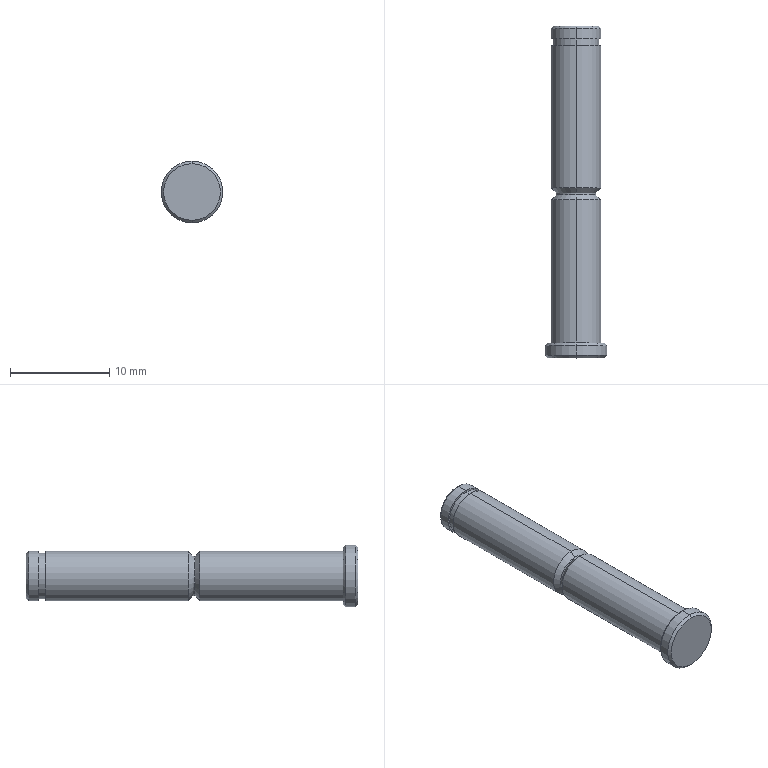Part | NX | features BREP 1 | 1 solid | 27 faces | box 6.2 x 33.4 x 6.2 mm | volume 662.792 mm3 | cylinder 12 | cone 10 | plane 5 | commonest cylinder face diameters 5 x6 4 x2 4.6 x2 6.2 x2
STEP:
#1=CARTESIAN_POINT('',(0.,33.4,2.25));
#2=VERTEX_POINT('',#1);
#3=CARTESIAN_POINT('',(0.,33.15,2.5));
#4=VERTEX_POINT('',#3);
#5=CARTESIAN_POINT('',(0.,33.15,2.5));
#6=DIRECTION('',(0.,-0.7071,0.7071));
#7=VECTOR('',#6,1000.);
#8=LINE('',#5,#7);
#9=EDGE_CURVE('',#2,#4,#8,.T.);
#10=ORIENTED_EDGE('',*,*,#9,.F.);
#11=CARTESIAN_POINT('',(0.,33.4,-2.25));
#12=VERTEX_POINT('',#11);
#13=CARTESIAN_POINT('',(0.,33.4,0.));
#14=DIRECTION('',(0.,1.,0.));
#15=DIRECTION('',(0.,0.,-1.));
#16=AXIS2_PLACEMENT_3D('',#13,#14,#15);
#17=CIRCLE('',#16,2.25);
#18=EDGE_CURVE('',#12,#2,#17,.T.);
#19=ORIENTED_EDGE('',*,*,#18,.F.);
#20=CARTESIAN_POINT('',(0.,33.15,-2.5));
#21=VERTEX_POINT('',#20);
#22=CARTESIAN_POINT('',(0.,33.15,-2.5));
#23=DIRECTION('',(0.,-0.7071,-0.7071));
#24=VECTOR('',#23,1000.);
#25=LINE('',#22,#24);
#26=EDGE_CURVE('',#12,#21,#25,.T.);
#27=ORIENTED_EDGE('',*,*,#26,.T.);
#28=CARTESIAN_POINT('',(0.,33.15,0.));
#29=DIRECTION('',(0.,-1.,0.));
#30=DIRECTION('',(0.,0.,-1.));
#31=AXIS2_PLACEMENT_3D('',#28,#29,#30);
#32=CIRCLE('',#31,2.5);
#33=EDGE_CURVE('',#4,#21,#32,.T.);
#34=ORIENTED_EDGE('',*,*,#33,.F.);
#35=EDGE_LOOP('',(#10,#19,#27,#34));
#36=FACE_BOUND('',#35,.T.);
#37=CARTESIAN_POINT('',(0.,33.15,0.));
#38=DIRECTION('',(0.,-1.,0.));
#39=DIRECTION('',(0.,0.,-1.));
#40=AXIS2_PLACEMENT_3D('',#37,#38,#39);
#41=CONICAL_SURFACE('',#40,2.5,0.7854);
#42=ADVANCED_FACE('',(#36),#41,.T.);
#43=CARTESIAN_POINT('',(0.,1.5,2.85));
#44=VERTEX_POINT('',#43);
#45=CARTESIAN_POINT('',(0.,1.25,3.1));
#46=VERTEX_POINT('',#45);
#47=CARTESIAN_POINT('',(0.,1.25,3.1));
#48=DIRECTION('',(0.,-0.7071,0.7071));
#49=VECTOR('',#48,1000.);
#50=LINE('',#47,#49);
#51=EDGE_CURVE('',#44,#46,#50,.T.);
#52=ORIENTED_EDGE('',*,*,#51,.F.);
#53=CARTESIAN_POINT('',(0.,1.5,-2.85));
#54=VERTEX_POINT('',#53);
#55=CARTESIAN_POINT('',(0.,1.5,0.));
#56=DIRECTION('',(0.,1.,0.));
#57=DIRECTION('',(0.,0.,-1.));
#58=AXIS2_PLACEMENT_3D('',#55,#56,#57);
#59=CIRCLE('',#58,2.85);
#60=EDGE_CURVE('',#54,#44,#59,.T.);
#61=ORIENTED_EDGE('',*,*,#60,.F.);
#62=CARTESIAN_POINT('',(0.,1.25,-3.1));
#63=VERTEX_POINT('',#62);
#64=CARTESIAN_POINT('',(0.,1.25,-3.1));
#65=DIRECTION('',(0.,-0.7071,-0.7071));
#66=VECTOR('',#65,1000.);
#67=LINE('',#64,#66);
#68=EDGE_CURVE('',#54,#63,#67,.T.);
#69=ORIENTED_EDGE('',*,*,#68,.T.);
#70=CARTESIAN_POINT('',(0.,1.25,0.));
#71=DIRECTION('',(0.,-1.,0.));
#72=DIRECTION('',(0.,0.,-1.));
#73=AXIS2_PLACEMENT_3D('',#70,#71,#72);
#74=CIRCLE('',#73,3.1);
#75=EDGE_CURVE('',#46,#63,#74,.T.);
#76=ORIENTED_EDGE('',*,*,#75,.F.);
#77=EDGE_LOOP('',(#52,#61,#69,#76));
#78=FACE_BOUND('',#77,.T.);
#79=CARTESIAN_POINT('',(0.,1.25,0.));
#80=DIRECTION('',(0.,-1.,0.));
#81=DIRECTION('',(0.,0.,-1.));
#82=AXIS2_PLACEMENT_3D('',#79,#80,#81);
#83=CONICAL_SURFACE('',#82,3.1,0.7854);
#84=ADVANCED_FACE('',(#78),#83,.T.);
#85=CARTESIAN_POINT('',(0.,0.25,-3.1));
#86=VERTEX_POINT('',#85);
#87=CARTESIAN_POINT('',(0.,0.,-2.85));
#88=VERTEX_POINT('',#87);
#89=CARTESIAN_POINT('',(0.,0.,-2.85));
#90=DIRECTION('',(0.,0.7071,-0.7071));
#91=VECTOR('',#90,1000.);
#92=LINE('',#89,#91);
#93=EDGE_CURVE('',#86,#88,#92,.F.);
#94=ORIENTED_EDGE('',*,*,#93,.T.);
#95=CARTESIAN_POINT('',(0.,0.,2.85));
#96=VERTEX_POINT('',#95);
#97=CARTESIAN_POINT('',(0.,0.,0.));
#98=DIRECTION('',(0.,-1.,0.));
#99=DIRECTION('',(0.,0.,1.));
#100=AXIS2_PLACEMENT_3D('',#97,#98,#99);
#101=CIRCLE('',#100,2.85);
#102=EDGE_CURVE('',#96,#88,#101,.T.);
#103=ORIENTED_EDGE('',*,*,#102,.F.);
#104=CARTESIAN_POINT('',(0.,0.25,3.1));
#105=VERTEX_POINT('',#104);
#106=CARTESIAN_POINT('',(0.,0.,2.85));
#107=DIRECTION('',(0.,0.7071,0.7071));
#108=VECTOR('',#107,1000.);
#109=LINE('',#106,#108);
#110=EDGE_CURVE('',#105,#96,#109,.F.);
#111=ORIENTED_EDGE('',*,*,#110,.F.);
#112=CARTESIAN_POINT('',(0.,0.25,0.));
#113=DIRECTION('',(0.,1.,0.));
#114=DIRECTION('',(0.,0.,1.));
#115=AXIS2_PLACEMENT_3D('',#112,#113,#114);
#116=CIRCLE('',#115,3.1);
#117=EDGE_CURVE('',#86,#105,#116,.T.);
#118=ORIENTED_EDGE('',*,*,#117,.F.);
#119=EDGE_LOOP('',(#94,#103,#111,#118));
#120=FACE_BOUND('',#119,.T.);
#121=CARTESIAN_POINT('',(0.,0.,0.));
#122=DIRECTION('',(0.,1.,0.));
#123=DIRECTION('',(0.,0.,1.));
#124=AXIS2_PLACEMENT_3D('',#121,#122,#123);
#125=CONICAL_SURFACE('',#124,2.85,0.7854);
#126=ADVANCED_FACE('',(#120),#125,.T.);
#127=ORIENTED_EDGE('',*,*,#18,.T.);
#128=CARTESIAN_POINT('',(0.,33.4,0.));
#129=DIRECTION('',(0.,1.,0.));
#130=DIRECTION('',(0.,0.,-1.));
#131=AXIS2_PLACEMENT_3D('',#128,#129,#130);
#132=CIRCLE('',#131,2.25);
#133=EDGE_CURVE('',#2,#12,#132,.T.);
#134=ORIENTED_EDGE('',*,*,#133,.T.);
#135=EDGE_LOOP('',(#127,#134));
#136=FACE_BOUND('',#135,.T.);
#137=CARTESIAN_POINT('',(-2.5,33.4,0.));
#138=DIRECTION('',(0.,-1.,0.));
#139=DIRECTION('',(0.,0.,-1.));
#140=AXIS2_PLACEMENT_3D('',#137,#138,#139);
#141=PLANE('',#140);
#142=ADVANCED_FACE('',(#136),#141,.F.);
#143=CARTESIAN_POINT('',(0.,32.1,2.5));
#144=VERTEX_POINT('',#143);
#145=CARTESIAN_POINT('',(0.,0.,2.5));
#146=DIRECTION('',(0.,-1.,0.));
#147=VECTOR('',#146,1000.);
#148=LINE('',#145,#147);
#149=EDGE_CURVE('',#4,#144,#148,.T.);
#150=ORIENTED_EDGE('',*,*,#149,.F.);
#151=ORIENTED_EDGE('',*,*,#33,.T.);
#152=CARTESIAN_POINT('',(0.,32.1,-2.5));
#153=VERTEX_POINT('',#152);
#154=CARTESIAN_POINT('',(0.,0.,-2.5));
#155=DIRECTION('',(0.,-1.,0.));
#156=VECTOR('',#155,1000.);
#157=LINE('',#154,#156);
#158=EDGE_CURVE('',#21,#153,#157,.T.);
#159=ORIENTED_EDGE('',*,*,#158,.T.);
#160=CARTESIAN_POINT('',(0.,32.1,0.));
#161=DIRECTION('',(0.,-1.,0.));
#162=DIRECTION('',(0.,0.,-1.));
#163=AXIS2_PLACEMENT_3D('',#160,#161,#162);
#164=CIRCLE('',#163,2.5);
#165=EDGE_CURVE('',#144,#153,#164,.T.);
#166=ORIENTED_EDGE('',*,*,#165,.F.);
#167=EDGE_LOOP('',(#150,#151,#159,#166));
#168=FACE_BOUND('',#167,.T.);
#169=CARTESIAN_POINT('',(0.,0.,0.));
#170=DIRECTION('',(0.,-1.,0.));
#171=DIRECTION('',(0.,0.,-1.));
#172=AXIS2_PLACEMENT_3D('',#169,#170,#171);
#173=CYLINDRICAL_SURFACE('',#172,2.5);
#174=ADVANCED_FACE('',(#168),#173,.T.);
#175=CARTESIAN_POINT('',(0.,32.1,0.));
#176=DIRECTION('',(0.,-1.,0.));
#177=DIRECTION('',(0.,0.,-1.));
#178=AXIS2_PLACEMENT_3D('',#175,#176,#177);
#179=CIRCLE('',#178,2.5);
#180=EDGE_CURVE('',#153,#144,#179,.T.);
#181=ORIENTED_EDGE('',*,*,#180,.T.);
#182=ORIENTED_EDGE('',*,*,#165,.T.);
#183=EDGE_LOOP('',(#181,#182));
#184=FACE_BOUND('',#183,.T.);
#185=CARTESIAN_POINT('',(0.,32.1,-2.3));
#186=VERTEX_POINT('',#185);
#187=CARTESIAN_POINT('',(0.,32.1,2.3));
#188=VERTEX_POINT('',#187);
#189=CARTESIAN_POINT('',(0.,32.1,0.));
#190=DIRECTION('',(0.,-1.,0.));
#191=DIRECTION('',(0.,0.,-1.));
#192=AXIS2_PLACEMENT_3D('',#189,#190,#191);
#193=CIRCLE('',#192,2.3);
#194=EDGE_CURVE('',#186,#188,#193,.T.);
#195=ORIENTED_EDGE('',*,*,#194,.F.);
#196=CARTESIAN_POINT('',(0.,32.1,0.));
#197=DIRECTION('',(0.,-1.,0.));
#198=DIRECTION('',(0.,0.,-1.));
#199=AXIS2_PLACEMENT_3D('',#196,#197,#198);
#200=CIRCLE('',#199,2.3);
#201=EDGE_CURVE('',#188,#186,#200,.T.);
#202=ORIENTED_EDGE('',*,*,#201,.F.);
#203=EDGE_LOOP('',(#195,#202));
#204=FACE_BOUND('',#203,.T.);
#205=CARTESIAN_POINT('',(-2.3,32.1,0.));
#206=DIRECTION('',(0.,1.,0.));
#207=DIRECTION('',(0.,0.,1.));
#208=AXIS2_PLACEMENT_3D('',#205,#206,#207);
#209=PLANE('',#208);
#210=ADVANCED_FACE('',(#184,#204),#209,.F.);
#211=CARTESIAN_POINT('',(0.,31.4,2.3));
#212=VERTEX_POINT('',#211);
#213=CARTESIAN_POINT('',(0.,0.,2.3));
#214=DIRECTION('',(0.,-1.,0.));
#215=VECTOR('',#214,1000.);
#216=LINE('',#213,#215);
#217=EDGE_CURVE('',#188,#212,#216,.T.);
#218=ORIENTED_EDGE('',*,*,#217,.F.);
#219=ORIENTED_EDGE('',*,*,#201,.T.);
#220=CARTESIAN_POINT('',(0.,31.4,-2.3));
#221=VERTEX_POINT('',#220);
#222=CARTESIAN_POINT('',(0.,0.,-2.3));
#223=DIRECTION('',(0.,-1.,0.));
#224=VECTOR('',#223,1000.);
#225=LINE('',#222,#224);
#226=EDGE_CURVE('',#186,#221,#225,.T.);
#227=ORIENTED_EDGE('',*,*,#226,.T.);
#228=CARTESIAN_POINT('',(0.,31.4,0.));
#229=DIRECTION('',(0.,-1.,0.));
#230=DIRECTION('',(0.,0.,-1.));
#231=AXIS2_PLACEMENT_3D('',#228,#229,#230);
#232=CIRCLE('',#231,2.3);
#233=EDGE_CURVE('',#212,#221,#232,.T.);
#234=ORIENTED_EDGE('',*,*,#233,.F.);
#235=EDGE_LOOP('',(#218,#219,#227,#234));
#236=FACE_BOUND('',#235,.T.);
#237=CARTESIAN_POINT('',(0.,0.,0.));
#238=DIRECTION('',(0.,-1.,0.));
#239=DIRECTION('',(0.,0.,-1.));
#240=AXIS2_PLACEMENT_3D('',#237,#238,#239);
#241=CYLINDRICAL_SURFACE('',#240,2.3);
#242=ADVANCED_FACE('',(#236),#241,.T.);
#243=CARTESIAN_POINT('',(0.,31.4,0.));
#244=DIRECTION('',(0.,-1.,0.));
#245=DIRECTION('',(0.,0.,-1.));
#246=AXIS2_PLACEMENT_3D('',#243,#244,#245);
#247=CIRCLE('',#246,2.3);
#248=EDGE_CURVE('',#221,#212,#247,.T.);
#249=ORIENTED_EDGE('',*,*,#248,.T.);
#250=ORIENTED_EDGE('',*,*,#233,.T.);
#251=EDGE_LOOP('',(#249,#250));
#252=FACE_BOUND('',#251,.T.);
#253=CARTESIAN_POINT('',(0.,31.4,-2.5));
#254=VERTEX_POINT('',#253);
#255=CARTESIAN_POINT('',(0.,31.4,2.5));
#256=VERTEX_POINT('',#255);
#257=CARTESIAN_POINT('',(0.,31.4,0.));
#258=DIRECTION('',(0.,-1.,0.));
#259=DIRECTION('',(0.,0.,-1.));
#260=AXIS2_PLACEMENT_3D('',#257,#258,#259);
#261=CIRCLE('',#260,2.5);
#262=EDGE_CURVE('',#254,#256,#261,.T.);
#263=ORIENTED_EDGE('',*,*,#262,.F.);
#264=CARTESIAN_POINT('',(0.,31.4,0.));
#265=DIRECTION('',(0.,-1.,0.));
#266=DIRECTION('',(0.,0.,-1.));
#267=AXIS2_PLACEMENT_3D('',#264,#265,#266);
#268=CIRCLE('',#267,2.5);
#269=EDGE_CURVE('',#256,#254,#268,.T.);
#270=ORIENTED_EDGE('',*,*,#269,.F.);
#271=EDGE_LOOP('',(#263,#270));
#272=FACE_BOUND('',#271,.T.);
#273=CARTESIAN_POINT('',(-2.5,31.4,0.));
#274=DIRECTION('',(0.,-1.,0.));
#275=DIRECTION('',(0.,0.,-1.));
#276=AXIS2_PLACEMENT_3D('',#273,#274,#275);
#277=PLANE('',#276);
#278=ADVANCED_FACE('',(#252,#272),#277,.F.);
#279=CARTESIAN_POINT('',(0.,17.1,2.5));
#280=VERTEX_POINT('',#279);
#281=CARTESIAN_POINT('',(0.,0.,2.5));
#282=DIRECTION('',(0.,-1.,0.));
#283=VECTOR('',#282,1000.);
#284=LINE('',#281,#283);
#285=EDGE_CURVE('',#256,#280,#284,.T.);
#286=ORIENTED_EDGE('',*,*,#285,.F.);
#287=ORIENTED_EDGE('',*,*,#269,.T.);
#288=CARTESIAN_POINT('',(0.,17.1,-2.5));
#289=VERTEX_POINT('',#288);
#290=CARTESIAN_POINT('',(0.,0.,-2.5));
#291=DIRECTION('',(0.,-1.,0.));
#292=VECTOR('',#291,1000.);
#293=LINE('',#290,#292);
#294=EDGE_CURVE('',#254,#289,#293,.T.);
#295=ORIENTED_EDGE('',*,*,#294,.T.);
#296=CARTESIAN_POINT('',(0.,17.1,0.));
#297=DIRECTION('',(0.,-1.,0.));
#298=DIRECTION('',(0.,0.,-1.));
#299=AXIS2_PLACEMENT_3D('',#296,#297,#298);
#300=CIRCLE('',#299,2.5);
#301=EDGE_CURVE('',#280,#289,#300,.T.);
#302=ORIENTED_EDGE('',*,*,#301,.F.);
#303=EDGE_LOOP('',(#286,#287,#295,#302));
#304=FACE_BOUND('',#303,.T.);
#305=CARTESIAN_POINT('',(0.,0.,0.));
#306=DIRECTION('',(0.,-1.,0.));
#307=DIRECTION('',(0.,0.,-1.));
#308=AXIS2_PLACEMENT_3D('',#305,#306,#307);
#309=CYLINDRICAL_SURFACE('',#308,2.5);
#310=ADVANCED_FACE('',(#304),#309,.T.);
#311=CARTESIAN_POINT('',(0.,16.6,-2.));
#312=VERTEX_POINT('',#311);
#313=CARTESIAN_POINT('',(0.,17.1,-2.5));
#314=DIRECTION('',(0.,0.7071,-0.7071));
#315=VECTOR('',#314,1000.);
#316=LINE('',#313,#315);
#317=EDGE_CURVE('',#289,#312,#316,.F.);
#318=ORIENTED_EDGE('',*,*,#317,.T.);
#319=CARTESIAN_POINT('',(0.,16.6,2.));
#320=VERTEX_POINT('',#319);
#321=CARTESIAN_POINT('',(0.,16.6,0.));
#322=DIRECTION('',(0.,-1.,0.));
#323=DIRECTION('',(0.,0.,-1.));
#324=AXIS2_PLACEMENT_3D('',#321,#322,#323);
#325=CIRCLE('',#324,2.);
#326=EDGE_CURVE('',#320,#312,#325,.T.);
#327=ORIENTED_EDGE('',*,*,#326,.F.);
#328=CARTESIAN_POINT('',(0.,17.1,2.5));
#329=DIRECTION('',(0.,0.7071,0.7071));
#330=VECTOR('',#329,1000.);
#331=LINE('',#328,#330);
#332=EDGE_CURVE('',#280,#320,#331,.F.);
#333=ORIENTED_EDGE('',*,*,#332,.F.);
#334=ORIENTED_EDGE('',*,*,#301,.T.);
#335=EDGE_LOOP('',(#318,#327,#333,#334));
#336=FACE_BOUND('',#335,.T.);
#337=CARTESIAN_POINT('',(0.,17.1,0.));
#338=DIRECTION('',(0.,1.,0.));
#339=DIRECTION('',(0.,0.,1.));
#340=AXIS2_PLACEMENT_3D('',#337,#338,#339);
#341=CONICAL_SURFACE('',#340,2.5,0.7854);
#342=ADVANCED_FACE('',(#336),#341,.T.);
#343=CARTESIAN_POINT('',(0.,16.4,2.));
#344=VERTEX_POINT('',#343);
#345=CARTESIAN_POINT('',(0.,0.,2.));
#346=DIRECTION('',(0.,-1.,0.));
#347=VECTOR('',#346,1000.);
#348=LINE('',#345,#347);
#349=EDGE_CURVE('',#320,#344,#348,.T.);
#350=ORIENTED_EDGE('',*,*,#349,.F.);
#351=ORIENTED_EDGE('',*,*,#326,.T.);
#352=CARTESIAN_POINT('',(0.,16.4,-2.));
#353=VERTEX_POINT('',#352);
#354=CARTESIAN_POINT('',(0.,0.,-2.));
#355=DIRECTION('',(0.,-1.,0.));
#356=VECTOR('',#355,1000.);
#357=LINE('',#354,#356);
#358=EDGE_CURVE('',#312,#353,#357,.T.);
#359=ORIENTED_EDGE('',*,*,#358,.T.);
#360=CARTESIAN_POINT('',(0.,16.4,0.));
#361=DIRECTION('',(0.,-1.,0.));
#362=DIRECTION('',(0.,0.,-1.));
#363=AXIS2_PLACEMENT_3D('',#360,#361,#362);
#364=CIRCLE('',#363,2.);
#365=EDGE_CURVE('',#344,#353,#364,.T.);
#366=ORIENTED_EDGE('',*,*,#365,.F.);
#367=EDGE_LOOP('',(#350,#351,#359,#366));
#368=FACE_BOUND('',#367,.T.);
#369=CARTESIAN_POINT('',(0.,0.,0.));
#370=DIRECTION('',(0.,-1.,0.));
#371=DIRECTION('',(0.,0.,-1.));
#372=AXIS2_PLACEMENT_3D('',#369,#370,#371);
#373=CYLINDRICAL_SURFACE('',#372,2.);
#374=ADVANCED_FACE('',(#368),#373,.T.);
#375=CARTESIAN_POINT('',(0.,15.9,2.5));
#376=VERTEX_POINT('',#375);
#377=CARTESIAN_POINT('',(0.,16.4,2.));
#378=DIRECTION('',(0.,-0.7071,0.7071));
#379=VECTOR('',#378,1000.);
#380=LINE('',#377,#379);
#381=EDGE_CURVE('',#344,#376,#380,.T.);
#382=ORIENTED_EDGE('',*,*,#381,.F.);
#383=ORIENTED_EDGE('',*,*,#365,.T.);
#384=CARTESIAN_POINT('',(0.,15.9,-2.5));
#385=VERTEX_POINT('',#384);
#386=CARTESIAN_POINT('',(0.,16.4,-2.));
#387=DIRECTION('',(0.,-0.7071,-0.7071));
#388=VECTOR('',#387,1000.);
#389=LINE('',#386,#388);
#390=EDGE_CURVE('',#353,#385,#389,.T.);
#391=ORIENTED_EDGE('',*,*,#390,.T.);
#392=CARTESIAN_POINT('',(0.,15.9,0.));
#393=DIRECTION('',(0.,-1.,0.));
#394=DIRECTION('',(0.,0.,-1.));
#395=AXIS2_PLACEMENT_3D('',#392,#393,#394);
#396=CIRCLE('',#395,2.5);
#397=EDGE_CURVE('',#376,#385,#396,.T.);
#398=ORIENTED_EDGE('',*,*,#397,.F.);
#399=EDGE_LOOP('',(#382,#383,#391,#398));
#400=FACE_BOUND('',#399,.T.);
#401=CARTESIAN_POINT('',(0.,16.4,0.));
#402=DIRECTION('',(0.,-1.,0.));
#403=DIRECTION('',(0.,0.,-1.));
#404=AXIS2_PLACEMENT_3D('',#401,#402,#403);
#405=CONICAL_SURFACE('',#404,2.,0.7854);
#406=ADVANCED_FACE('',(#400),#405,.T.);
#407=CARTESIAN_POINT('',(0.,1.5,2.5));
#408=VERTEX_POINT('',#407);
#409=CARTESIAN_POINT('',(0.,0.,2.5));
#410=DIRECTION('',(0.,-1.,0.));
#411=VECTOR('',#410,1000.);
#412=LINE('',#409,#411);
#413=EDGE_CURVE('',#376,#408,#412,.T.);
#414=ORIENTED_EDGE('',*,*,#413,.F.);
#415=ORIENTED_EDGE('',*,*,#397,.T.);
#416=CARTESIAN_POINT('',(0.,1.5,-2.5));
#417=VERTEX_POINT('',#416);
#418=CARTESIAN_POINT('',(0.,0.,-2.5));
#419=DIRECTION('',(0.,-1.,0.));
#420=VECTOR('',#419,1000.);
#421=LINE('',#418,#420);
#422=EDGE_CURVE('',#385,#417,#421,.T.);
#423=ORIENTED_EDGE('',*,*,#422,.T.);
#424=CARTESIAN_POINT('',(0.,1.5,0.));
#425=DIRECTION('',(0.,-1.,0.));
#426=DIRECTION('',(0.,0.,-1.));
#427=AXIS2_PLACEMENT_3D('',#424,#425,#426);
#428=CIRCLE('',#427,2.5);
#429=EDGE_CURVE('',#408,#417,#428,.T.);
#430=ORIENTED_EDGE('',*,*,#429,.F.);
#431=EDGE_LOOP('',(#414,#415,#423,#430));
#432=FACE_BOUND('',#431,.T.);
#433=CARTESIAN_POINT('',(0.,0.,0.));
#434=DIRECTION('',(0.,-1.,0.));
#435=DIRECTION('',(0.,0.,-1.));
#436=AXIS2_PLACEMENT_3D('',#433,#434,#435);
#437=CYLINDRICAL_SURFACE('',#436,2.5);
#438=ADVANCED_FACE('',(#432),#437,.T.);
#439=CARTESIAN_POINT('',(0.,1.5,0.));
#440=DIRECTION('',(0.,-1.,0.));
#441=DIRECTION('',(0.,0.,-1.));
#442=AXIS2_PLACEMENT_3D('',#439,#440,#441);
#443=CIRCLE('',#442,2.5);
#444=EDGE_CURVE('',#417,#408,#443,.T.);
#445=ORIENTED_EDGE('',*,*,#444,.T.);
#446=ORIENTED_EDGE('',*,*,#429,.T.);
#447=EDGE_LOOP('',(#445,#446));
#448=FACE_BOUND('',#447,.T.);
#449=ORIENTED_EDGE('',*,*,#60,.T.);
#450=CARTESIAN_POINT('',(0.,1.5,0.));
#451=DIRECTION('',(0.,1.,0.));
#452=DIRECTION('',(0.,0.,-1.));
#453=AXIS2_PLACEMENT_3D('',#450,#451,#452);
#454=CIRCLE('',#453,2.85);
#455=EDGE_CURVE('',#44,#54,#454,.T.);
#456=ORIENTED_EDGE('',*,*,#455,.T.);
#457=EDGE_LOOP('',(#449,#456));
#458=FACE_BOUND('',#457,.T.);
#459=CARTESIAN_POINT('',(-3.1,1.5,0.));
#460=DIRECTION('',(0.,-1.,0.));
#461=DIRECTION('',(0.,0.,-1.));
#462=AXIS2_PLACEMENT_3D('',#459,#460,#461);
#463=PLANE('',#462);
#464=ADVANCED_FACE('',(#448,#458),#463,.F.);
#465=CARTESIAN_POINT('',(0.,0.,3.1));
#466=DIRECTION('',(0.,-1.,0.));
#467=VECTOR('',#466,1000.);
#468=LINE('',#465,#467);
#469=EDGE_CURVE('',#46,#105,#468,.T.);
#470=ORIENTED_EDGE('',*,*,#469,.F.);
#471=ORIENTED_EDGE('',*,*,#75,.T.);
#472=CARTESIAN_POINT('',(0.,0.,-3.1));
#473=DIRECTION('',(0.,-1.,0.));
#474=VECTOR('',#473,1000.);
#475=LINE('',#472,#474);
#476=EDGE_CURVE('',#63,#86,#475,.T.);
#477=ORIENTED_EDGE('',*,*,#476,.T.);
#478=ORIENTED_EDGE('',*,*,#117,.T.);
#479=EDGE_LOOP('',(#470,#471,#477,#478));
#480=FACE_BOUND('',#479,.T.);
#481=CARTESIAN_POINT('',(0.,0.,0.));
#482=DIRECTION('',(0.,-1.,0.));
#483=DIRECTION('',(0.,0.,-1.));
#484=AXIS2_PLACEMENT_3D('',#481,#482,#483);
#485=CYLINDRICAL_SURFACE('',#484,3.1);
#486=ADVANCED_FACE('',(#480),#485,.T.);
#487=ORIENTED_EDGE('',*,*,#102,.T.);
#488=CARTESIAN_POINT('',(0.,0.,0.));
#489=DIRECTION('',(0.,-1.,0.));
#490=DIRECTION('',(0.,0.,1.));
#491=AXIS2_PLACEMENT_3D('',#488,#489,#490);
#492=CIRCLE('',#491,2.85);
#493=EDGE_CURVE('',#88,#96,#492,.T.);
#494=ORIENTED_EDGE('',*,*,#493,.T.);
#495=EDGE_LOOP('',(#487,#494));
#496=FACE_BOUND('',#495,.T.);
#497=CARTESIAN_POINT('',(0.,0.,0.));
#498=DIRECTION('',(0.,1.,0.));
#499=DIRECTION('',(0.,0.,1.));
#500=AXIS2_PLACEMENT_3D('',#497,#498,#499);
#501=PLANE('',#500);
#502=ADVANCED_FACE('',(#496),#501,.F.);
#503=CARTESIAN_POINT('',(0.,1.25,0.));
#504=DIRECTION('',(0.,-1.,0.));
#505=DIRECTION('',(0.,0.,-1.));
#506=AXIS2_PLACEMENT_3D('',#503,#504,#505);
#507=CIRCLE('',#506,3.1);
#508=EDGE_CURVE('',#63,#46,#507,.T.);
#509=ORIENTED_EDGE('',*,*,#508,.T.);
#510=ORIENTED_EDGE('',*,*,#469,.T.);
#511=CARTESIAN_POINT('',(0.,0.25,0.));
#512=DIRECTION('',(0.,1.,0.));
#513=DIRECTION('',(0.,0.,1.));
#514=AXIS2_PLACEMENT_3D('',#511,#512,#513);
#515=CIRCLE('',#514,3.1);
#516=EDGE_CURVE('',#105,#86,#515,.T.);
#517=ORIENTED_EDGE('',*,*,#516,.T.);
#518=ORIENTED_EDGE('',*,*,#476,.F.);
#519=EDGE_LOOP('',(#509,#510,#517,#518));
#520=FACE_BOUND('',#519,.T.);
#521=CARTESIAN_POINT('',(0.,0.,0.));
#522=DIRECTION('',(0.,-1.,0.));
#523=DIRECTION('',(0.,0.,-1.));
#524=AXIS2_PLACEMENT_3D('',#521,#522,#523);
#525=CYLINDRICAL_SURFACE('',#524,3.1);
#526=ADVANCED_FACE('',(#520),#525,.T.);
#527=CARTESIAN_POINT('',(0.,15.9,0.));
#528=DIRECTION('',(0.,-1.,0.));
#529=DIRECTION('',(0.,0.,-1.));
#530=AXIS2_PLACEMENT_3D('',#527,#528,#529);
#531=CIRCLE('',#530,2.5);
#532=EDGE_CURVE('',#385,#376,#531,.T.);
#533=ORIENTED_EDGE('',*,*,#532,.T.);
#534=ORIENTED_EDGE('',*,*,#413,.T.);
#535=ORIENTED_EDGE('',*,*,#444,.F.);
#536=ORIENTED_EDGE('',*,*,#422,.F.);
#537=EDGE_LOOP('',(#533,#534,#535,#536));
#538=FACE_BOUND('',#537,.T.);
#539=CARTESIAN_POINT('',(0.,0.,0.));
#540=DIRECTION('',(0.,-1.,0.));
#541=DIRECTION('',(0.,0.,-1.));
#542=AXIS2_PLACEMENT_3D('',#539,#540,#541);
#543=CYLINDRICAL_SURFACE('',#542,2.5);
#544=ADVANCED_FACE('',(#538),#543,.T.);
#545=CARTESIAN_POINT('',(0.,16.4,0.));
#546=DIRECTION('',(0.,-1.,0.));
#547=DIRECTION('',(0.,0.,-1.));
#548=AXIS2_PLACEMENT_3D('',#545,#546,#547);
#549=CIRCLE('',#548,2.);
#550=EDGE_CURVE('',#353,#344,#549,.T.);
#551=ORIENTED_EDGE('',*,*,#550,.T.);
#552=ORIENTED_EDGE('',*,*,#381,.T.);
#553=ORIENTED_EDGE('',*,*,#532,.F.);
#554=ORIENTED_EDGE('',*,*,#390,.F.);
#555=EDGE_LOOP('',(#551,#552,#553,#554));
#556=FACE_BOUND('',#555,.T.);
#557=CARTESIAN_POINT('',(0.,16.4,0.));
#558=DIRECTION('',(0.,-1.,0.));
#559=DIRECTION('',(0.,0.,-1.));
#560=AXIS2_PLACEMENT_3D('',#557,#558,#559);
#561=CONICAL_SURFACE('',#560,2.,0.7854);
#562=ADVANCED_FACE('',(#556),#561,.T.);
#563=CARTESIAN_POINT('',(0.,16.6,0.));
#564=DIRECTION('',(0.,-1.,0.));
#565=DIRECTION('',(0.,0.,-1.));
#566=AXIS2_PLACEMENT_3D('',#563,#564,#565);
#567=CIRCLE('',#566,2.);
#568=EDGE_CURVE('',#312,#320,#567,.T.);
#569=ORIENTED_EDGE('',*,*,#568,.T.);
#570=ORIENTED_EDGE('',*,*,#349,.T.);
#571=ORIENTED_EDGE('',*,*,#550,.F.);
#572=ORIENTED_EDGE('',*,*,#358,.F.);
#573=EDGE_LOOP('',(#569,#570,#571,#572));
#574=FACE_BOUND('',#573,.T.);
#575=CARTESIAN_POINT('',(0.,0.,0.));
#576=DIRECTION('',(0.,-1.,0.));
#577=DIRECTION('',(0.,0.,-1.));
#578=AXIS2_PLACEMENT_3D('',#575,#576,#577);
#579=CYLINDRICAL_SURFACE('',#578,2.);
#580=ADVANCED_FACE('',(#574),#579,.T.);
#581=ORIENTED_EDGE('',*,*,#568,.F.);
#582=ORIENTED_EDGE('',*,*,#317,.F.);
#583=CARTESIAN_POINT('',(0.,17.1,0.));
#584=DIRECTION('',(0.,-1.,0.));
#585=DIRECTION('',(0.,0.,-1.));
#586=AXIS2_PLACEMENT_3D('',#583,#584,#585);
#587=CIRCLE('',#586,2.5);
#588=EDGE_CURVE('',#289,#280,#587,.T.);
#589=ORIENTED_EDGE('',*,*,#588,.T.);
#590=ORIENTED_EDGE('',*,*,#332,.T.);
#591=EDGE_LOOP('',(#581,#582,#589,#590));
#592=FACE_BOUND('',#591,.T.);
#593=CARTESIAN_POINT('',(0.,17.1,0.));
#594=DIRECTION('',(0.,1.,0.));
#595=DIRECTION('',(0.,0.,1.));
#596=AXIS2_PLACEMENT_3D('',#593,#594,#595);
#597=CONICAL_SURFACE('',#596,2.5,0.7854);
#598=ADVANCED_FACE('',(#592),#597,.T.);
#599=ORIENTED_EDGE('',*,*,#262,.T.);
#600=ORIENTED_EDGE('',*,*,#285,.T.);
#601=ORIENTED_EDGE('',*,*,#588,.F.);
#602=ORIENTED_EDGE('',*,*,#294,.F.);
#603=EDGE_LOOP('',(#599,#600,#601,#602));
#604=FACE_BOUND('',#603,.T.);
#605=CARTESIAN_POINT('',(0.,0.,0.));
#606=DIRECTION('',(0.,-1.,0.));
#607=DIRECTION('',(0.,0.,-1.));
#608=AXIS2_PLACEMENT_3D('',#605,#606,#607);
#609=CYLINDRICAL_SURFACE('',#608,2.5);
#610=ADVANCED_FACE('',(#604),#609,.T.);
#611=ORIENTED_EDGE('',*,*,#194,.T.);
#612=ORIENTED_EDGE('',*,*,#217,.T.);
#613=ORIENTED_EDGE('',*,*,#248,.F.);
#614=ORIENTED_EDGE('',*,*,#226,.F.);
#615=EDGE_LOOP('',(#611,#612,#613,#614));
#616=FACE_BOUND('',#615,.T.);
#617=CARTESIAN_POINT('',(0.,0.,0.));
#618=DIRECTION('',(0.,-1.,0.));
#619=DIRECTION('',(0.,0.,-1.));
#620=AXIS2_PLACEMENT_3D('',#617,#618,#619);
#621=CYLINDRICAL_SURFACE('',#620,2.3);
#622=ADVANCED_FACE('',(#616),#621,.T.);
#623=CARTESIAN_POINT('',(0.,33.15,0.));
#624=DIRECTION('',(0.,-1.,0.));
#625=DIRECTION('',(0.,0.,-1.));
#626=AXIS2_PLACEMENT_3D('',#623,#624,#625);
#627=CIRCLE('',#626,2.5);
#628=EDGE_CURVE('',#21,#4,#627,.T.);
#629=ORIENTED_EDGE('',*,*,#628,.T.);
#630=ORIENTED_EDGE('',*,*,#149,.T.);
#631=ORIENTED_EDGE('',*,*,#180,.F.);
#632=ORIENTED_EDGE('',*,*,#158,.F.);
#633=EDGE_LOOP('',(#629,#630,#631,#632));
#634=FACE_BOUND('',#633,.T.);
#635=CARTESIAN_POINT('',(0.,0.,0.));
#636=DIRECTION('',(0.,-1.,0.));
#637=DIRECTION('',(0.,0.,-1.));
#638=AXIS2_PLACEMENT_3D('',#635,#636,#637);
#639=CYLINDRICAL_SURFACE('',#638,2.5);
#640=ADVANCED_FACE('',(#634),#639,.T.);
#641=ORIENTED_EDGE('',*,*,#493,.F.);
#642=ORIENTED_EDGE('',*,*,#93,.F.);
#643=ORIENTED_EDGE('',*,*,#516,.F.);
#644=ORIENTED_EDGE('',*,*,#110,.T.);
#645=EDGE_LOOP('',(#641,#642,#643,#644));
#646=FACE_BOUND('',#645,.T.);
#647=CARTESIAN_POINT('',(0.,0.,0.));
#648=DIRECTION('',(0.,1.,0.));
#649=DIRECTION('',(0.,0.,1.));
#650=AXIS2_PLACEMENT_3D('',#647,#648,#649);
#651=CONICAL_SURFACE('',#650,2.85,0.7854);
#652=ADVANCED_FACE('',(#646),#651,.T.);
#653=ORIENTED_EDGE('',*,*,#455,.F.);
#654=ORIENTED_EDGE('',*,*,#51,.T.);
#655=ORIENTED_EDGE('',*,*,#508,.F.);
#656=ORIENTED_EDGE('',*,*,#68,.F.);
#657=EDGE_LOOP('',(#653,#654,#655,#656));
#658=FACE_BOUND('',#657,.T.);
#659=CARTESIAN_POINT('',(0.,1.25,0.));
#660=DIRECTION('',(0.,-1.,0.));
#661=DIRECTION('',(0.,0.,-1.));
#662=AXIS2_PLACEMENT_3D('',#659,#660,#661);
#663=CONICAL_SURFACE('',#662,3.1,0.7854);
#664=ADVANCED_FACE('',(#658),#663,.T.);
#665=ORIENTED_EDGE('',*,*,#133,.F.);
#666=ORIENTED_EDGE('',*,*,#9,.T.);
#667=ORIENTED_EDGE('',*,*,#628,.F.);
#668=ORIENTED_EDGE('',*,*,#26,.F.);
#669=EDGE_LOOP('',(#665,#666,#667,#668));
#670=FACE_BOUND('',#669,.T.);
#671=CARTESIAN_POINT('',(0.,33.15,0.));
#672=DIRECTION('',(0.,-1.,0.));
#673=DIRECTION('',(0.,0.,-1.));
#674=AXIS2_PLACEMENT_3D('',#671,#672,#673);
#675=CONICAL_SURFACE('',#674,2.5,0.7854);
#676=ADVANCED_FACE('',(#670),#675,.T.);
#677=CLOSED_SHELL('',(#42,#84,#126,#142,#174,#210,#242,#278,#310,#342,#374,#406,#438,#464,#486,#502,#526,#544,#562,#580,#598,#610,#622,#640,#652,#664,#676));
#678=MANIFOLD_SOLID_BREP('',#677);
#679=(LENGTH_UNIT()NAMED_UNIT(*)SI_UNIT(.MILLI.,.METRE.));
#680=UNCERTAINTY_MEASURE_WITH_UNIT(LENGTH_MEASURE(0.00001),#679,'','');
#681=(NAMED_UNIT(*)PLANE_ANGLE_UNIT()SI_UNIT($,.RADIAN.));
#682=(NAMED_UNIT(*)SI_UNIT($,.STERADIAN.)SOLID_ANGLE_UNIT());
#683=(GEOMETRIC_REPRESENTATION_CONTEXT(3)GLOBAL_UNCERTAINTY_ASSIGNED_CONTEXT((#680))GLOBAL_UNIT_ASSIGNED_CONTEXT((#679,#681,#682))REPRESENTATION_CONTEXT('',''));
#684=ADVANCED_BREP_SHAPE_REPRESENTATION('',(#678),#683);